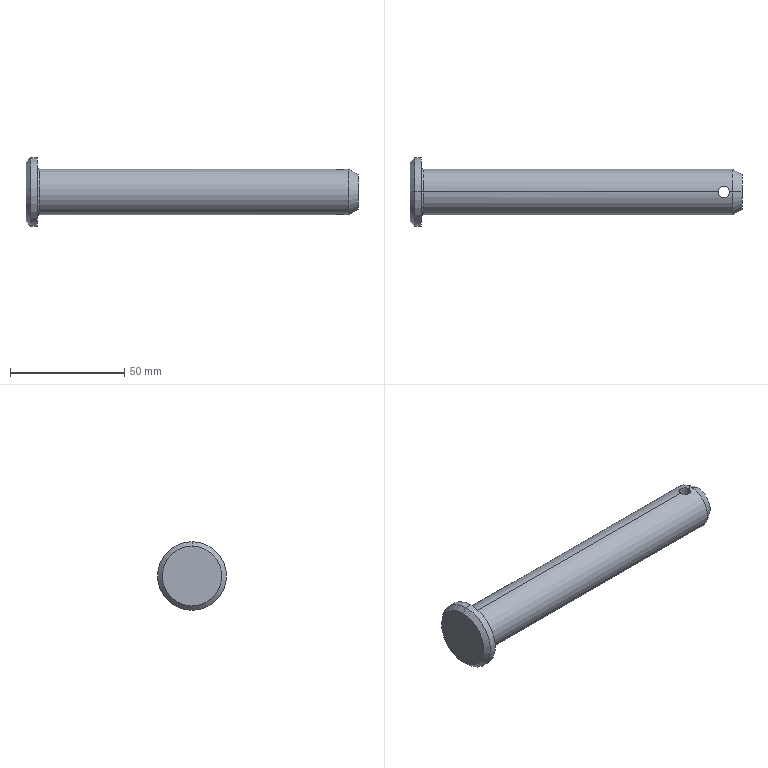Part | SolidWorks | features Chamfer 1, Fillet 1, ICE 1, Revolution 1 | 1 solid | 15 faces | box 145 x 30 x 30 mm | volume 46693 mm3 | cylinder 6 | cone 4 | plane 3 | torus 2 | commonest cylinder face diameters 5 x2 20 x2 30 x2
STEP:
#1=CARTESIAN_POINT('',(145.,0.,-7.691));
#2=VERTEX_POINT('',#1);
#3=CARTESIAN_POINT('',(145.,0.,7.691));
#4=VERTEX_POINT('',#3);
#5=CARTESIAN_POINT('',(145.,0.,0.));
#6=DIRECTION('',(1.,0.,0.));
#7=DIRECTION('',(0.,0.,-1.));
#8=AXIS2_PLACEMENT_3D('',#5,#6,#7);
#9=CIRCLE('',#8,7.691);
#10=EDGE_CURVE('',#2,#4,#9,.T.);
#11=ORIENTED_EDGE('',*,*,#10,.F.);
#12=CARTESIAN_POINT('',(141.,0.,-10.));
#13=VERTEX_POINT('',#12);
#14=CARTESIAN_POINT('',(145.,0.,-7.691));
#15=DIRECTION('',(-0.866,0.,-0.5));
#16=VECTOR('',#15,1000.);
#17=LINE('',#14,#16);
#18=EDGE_CURVE('',#2,#13,#17,.T.);
#19=ORIENTED_EDGE('',*,*,#18,.T.);
#20=CARTESIAN_POINT('',(141.,0.,10.));
#21=VERTEX_POINT('',#20);
#22=CARTESIAN_POINT('',(141.,0.,0.));
#23=DIRECTION('',(-1.,0.,0.));
#24=DIRECTION('',(0.,0.,-1.));
#25=AXIS2_PLACEMENT_3D('',#22,#23,#24);
#26=CIRCLE('',#25,10.);
#27=EDGE_CURVE('',#21,#13,#26,.T.);
#28=ORIENTED_EDGE('',*,*,#27,.F.);
#29=CARTESIAN_POINT('',(145.,0.,7.691));
#30=DIRECTION('',(-0.866,0.,0.5));
#31=VECTOR('',#30,1000.);
#32=LINE('',#29,#31);
#33=EDGE_CURVE('',#4,#21,#32,.T.);
#34=ORIENTED_EDGE('',*,*,#33,.F.);
#35=EDGE_LOOP('',(#11,#19,#28,#34));
#36=FACE_OUTER_BOUND('',#35,.T.);
#37=CARTESIAN_POINT('',(145.,0.,0.));
#38=DIRECTION('',(-1.,0.,0.));
#39=DIRECTION('',(0.,0.,1.));
#40=AXIS2_PLACEMENT_3D('',#37,#38,#39);
#41=CONICAL_SURFACE('',#40,7.691,0.5236);
#42=ADVANCED_FACE('',(#36),#41,.T.);
#43=CARTESIAN_POINT('',(6.,0.,10.));
#44=VERTEX_POINT('',#43);
#45=CARTESIAN_POINT('',(6.,0.,-10.));
#46=VERTEX_POINT('',#45);
#47=CARTESIAN_POINT('',(6.,0.,0.));
#48=DIRECTION('',(1.,0.,0.));
#49=DIRECTION('',(0.,0.,-1.));
#50=AXIS2_PLACEMENT_3D('',#47,#48,#49);
#51=CIRCLE('',#50,10.);
#52=EDGE_CURVE('',#44,#46,#51,.T.);
#53=ORIENTED_EDGE('',*,*,#52,.F.);
#54=CARTESIAN_POINT('',(5.,0.,11.));
#55=VERTEX_POINT('',#54);
#56=CARTESIAN_POINT('',(6.,0.,11.));
#57=DIRECTION('',(0.,1.,0.));
#58=DIRECTION('',(0.,0.,1.));
#59=AXIS2_PLACEMENT_3D('',#56,#57,#58);
#60=CIRCLE('',#59,1.);
#61=EDGE_CURVE('',#44,#55,#60,.T.);
#62=ORIENTED_EDGE('',*,*,#61,.T.);
#63=CARTESIAN_POINT('',(5.,0.,-11.));
#64=VERTEX_POINT('',#63);
#65=CARTESIAN_POINT('',(5.,0.,0.));
#66=DIRECTION('',(-1.,0.,0.));
#67=DIRECTION('',(0.,0.,-1.));
#68=AXIS2_PLACEMENT_3D('',#65,#66,#67);
#69=CIRCLE('',#68,11.);
#70=EDGE_CURVE('',#64,#55,#69,.T.);
#71=ORIENTED_EDGE('',*,*,#70,.F.);
#72=CARTESIAN_POINT('',(6.,0.,-11.));
#73=DIRECTION('',(0.,-1.,0.));
#74=DIRECTION('',(0.,0.,-1.));
#75=AXIS2_PLACEMENT_3D('',#72,#73,#74);
#76=CIRCLE('',#75,1.);
#77=EDGE_CURVE('',#46,#64,#76,.T.);
#78=ORIENTED_EDGE('',*,*,#77,.F.);
#79=EDGE_LOOP('',(#53,#62,#71,#78));
#80=FACE_OUTER_BOUND('',#79,.T.);
#81=CARTESIAN_POINT('',(6.,0.,0.));
#82=DIRECTION('',(1.,0.,0.));
#83=DIRECTION('',(0.,0.,-1.));
#84=AXIS2_PLACEMENT_3D('',#81,#82,#83);
#85=TOROIDAL_SURFACE('',#84,11.,1.);
#86=ADVANCED_FACE('',(#80),#85,.F.);
#87=CARTESIAN_POINT('',(139.5,0.,-10.));
#88=VERTEX_POINT('',#87);
#89=CARTESIAN_POINT('',(134.5,0.,-10.));
#90=VERTEX_POINT('',#89);
#91=CARTESIAN_POINT('',(139.5,0.,-10.));
#92=CARTESIAN_POINT('',(139.5,-0.327,-10.));
#93=CARTESIAN_POINT('',(139.434,-0.6572,-9.983));
#94=CARTESIAN_POINT('',(139.247,-1.109,-9.939));
#95=CARTESIAN_POINT('',(139.168,-1.255,-9.922));
#96=CARTESIAN_POINT('',(138.987,-1.526,-9.884));
#97=CARTESIAN_POINT('',(138.884,-1.652,-9.863));
#98=CARTESIAN_POINT('',(138.653,-1.882,-9.822));
#99=CARTESIAN_POINT('',(138.525,-1.987,-9.801));
#100=CARTESIAN_POINT('',(138.255,-2.168,-9.763));
#101=CARTESIAN_POINT('',(138.112,-2.245,-9.745));
#102=CARTESIAN_POINT('',(137.808,-2.372,-9.715));
#103=CARTESIAN_POINT('',(137.651,-2.419,-9.703));
#104=CARTESIAN_POINT('',(137.331,-2.483,-9.687));
#105=CARTESIAN_POINT('',(137.166,-2.5,-9.682));
#106=CARTESIAN_POINT('',(136.836,-2.5,-9.682));
#107=CARTESIAN_POINT('',(136.673,-2.484,-9.687));
#108=CARTESIAN_POINT('',(136.352,-2.42,-9.703));
#109=CARTESIAN_POINT('',(136.193,-2.372,-9.715));
#110=CARTESIAN_POINT('',(135.891,-2.247,-9.745));
#111=CARTESIAN_POINT('',(135.747,-2.17,-9.762));
#112=CARTESIAN_POINT('',(135.475,-1.988,-9.801));
#113=CARTESIAN_POINT('',(135.348,-1.883,-9.822));
#114=CARTESIAN_POINT('',(135.118,-1.654,-9.863));
#115=CARTESIAN_POINT('',(135.014,-1.527,-9.884));
#116=CARTESIAN_POINT('',(134.832,-1.255,-9.922));
#117=CARTESIAN_POINT('',(134.755,-1.112,-9.939));
#118=CARTESIAN_POINT('',(134.629,-0.8107,-9.968));
#119=CARTESIAN_POINT('',(134.581,-0.6515,-9.98));
#120=CARTESIAN_POINT('',(134.516,-0.3293,-9.996));
#121=CARTESIAN_POINT('',(134.5,-0.1658,-10.));
#122=CARTESIAN_POINT('',(134.5,0.,-10.));
#123=B_SPLINE_CURVE_WITH_KNOTS('',3,(#91,#92,#93,#94,#95,#96,#97,#98,#99,#100,#101,#102,#103,#104,#105,#106,#107,#108,#109,#110,#111,#112,#113,#114,#115,#116,#117,#118,#119,#120,#121,#122),.UNSPECIFIED.,.F.,.F.,(4,2,2,2,2,2,2,2,2,2,2,2,2,2,2,4),(0.007847,0.008828,0.009318,0.009809,0.0103,0.01079,0.01128,0.01177,0.01226,0.01275,0.01324,0.01373,0.01422,0.01471,0.0152,0.01569),.UNSPECIFIED.);
#124=EDGE_CURVE('',#88,#90,#123,.T.);
#125=ORIENTED_EDGE('',*,*,#124,.T.);
#126=CARTESIAN_POINT('',(134.5,0.,10.));
#127=VERTEX_POINT('',#126);
#128=CARTESIAN_POINT('',(134.5,0.,-15.));
#129=DIRECTION('',(0.,0.,1.));
#130=VECTOR('',#129,1000.);
#131=LINE('',#128,#130);
#132=EDGE_CURVE('',#90,#127,#131,.T.);
#133=ORIENTED_EDGE('',*,*,#132,.T.);
#134=CARTESIAN_POINT('',(139.5,0.,10.));
#135=VERTEX_POINT('',#134);
#136=CARTESIAN_POINT('',(134.5,0.,10.));
#137=CARTESIAN_POINT('',(134.5,-0.327,10.));
#138=CARTESIAN_POINT('',(134.566,-0.6572,9.983));
#139=CARTESIAN_POINT('',(134.753,-1.109,9.939));
#140=CARTESIAN_POINT('',(134.832,-1.255,9.922));
#141=CARTESIAN_POINT('',(135.013,-1.526,9.884));
#142=CARTESIAN_POINT('',(135.116,-1.652,9.863));
#143=CARTESIAN_POINT('',(135.347,-1.882,9.822));
#144=CARTESIAN_POINT('',(135.475,-1.987,9.801));
#145=CARTESIAN_POINT('',(135.745,-2.168,9.763));
#146=CARTESIAN_POINT('',(135.888,-2.245,9.745));
#147=CARTESIAN_POINT('',(136.192,-2.372,9.715));
#148=CARTESIAN_POINT('',(136.349,-2.419,9.703));
#149=CARTESIAN_POINT('',(136.669,-2.483,9.687));
#150=CARTESIAN_POINT('',(136.834,-2.5,9.682));
#151=CARTESIAN_POINT('',(137.164,-2.5,9.682));
#152=CARTESIAN_POINT('',(137.327,-2.484,9.687));
#153=CARTESIAN_POINT('',(137.648,-2.42,9.703));
#154=CARTESIAN_POINT('',(137.807,-2.372,9.715));
#155=CARTESIAN_POINT('',(138.109,-2.247,9.745));
#156=CARTESIAN_POINT('',(138.253,-2.17,9.762));
#157=CARTESIAN_POINT('',(138.525,-1.988,9.801));
#158=CARTESIAN_POINT('',(138.652,-1.883,9.822));
#159=CARTESIAN_POINT('',(138.882,-1.654,9.863));
#160=CARTESIAN_POINT('',(138.986,-1.527,9.884));
#161=CARTESIAN_POINT('',(139.168,-1.255,9.922));
#162=CARTESIAN_POINT('',(139.245,-1.112,9.939));
#163=CARTESIAN_POINT('',(139.371,-0.8107,9.968));
#164=CARTESIAN_POINT('',(139.419,-0.6515,9.98));
#165=CARTESIAN_POINT('',(139.484,-0.3293,9.996));
#166=CARTESIAN_POINT('',(139.5,-0.1658,10.));
#167=CARTESIAN_POINT('',(139.5,0.,10.));
#168=B_SPLINE_CURVE_WITH_KNOTS('',3,(#136,#137,#138,#139,#140,#141,#142,#143,#144,#145,#146,#147,#148,#149,#150,#151,#152,#153,#154,#155,#156,#157,#158,#159,#160,#161,#162,#163,#164,#165,#166,#167),.UNSPECIFIED.,.F.,.F.,(4,2,2,2,2,2,2,2,2,2,2,2,2,2,2,4),(0.007847,0.008828,0.009318,0.009809,0.0103,0.01079,0.01128,0.01177,0.01226,0.01275,0.01324,0.01373,0.01422,0.01471,0.0152,0.01569),.UNSPECIFIED.);
#169=EDGE_CURVE('',#127,#135,#168,.T.);
#170=ORIENTED_EDGE('',*,*,#169,.T.);
#171=CARTESIAN_POINT('',(139.5,0.,-15.));
#172=DIRECTION('',(0.,0.,1.));
#173=VECTOR('',#172,1000.);
#174=LINE('',#171,#173);
#175=EDGE_CURVE('',#88,#135,#174,.T.);
#176=ORIENTED_EDGE('',*,*,#175,.F.);
#177=EDGE_LOOP('',(#125,#133,#170,#176));
#178=FACE_OUTER_BOUND('',#177,.T.);
#179=CARTESIAN_POINT('',(137.,0.,-15.));
#180=DIRECTION('',(0.,0.,1.));
#181=DIRECTION('',(1.,0.,0.));
#182=AXIS2_PLACEMENT_3D('',#179,#180,#181);
#183=CYLINDRICAL_SURFACE('',#182,2.5);
#184=ADVANCED_FACE('',(#178),#183,.F.);
#185=CARTESIAN_POINT('',(6.,0.,0.));
#186=DIRECTION('',(1.,0.,0.));
#187=DIRECTION('',(0.,0.,-1.));
#188=AXIS2_PLACEMENT_3D('',#185,#186,#187);
#189=CIRCLE('',#188,10.);
#190=EDGE_CURVE('',#46,#44,#189,.T.);
#191=ORIENTED_EDGE('',*,*,#190,.T.);
#192=CARTESIAN_POINT('',(0.,0.,10.));
#193=DIRECTION('',(1.,0.,0.));
#194=VECTOR('',#193,1000.);
#195=LINE('',#192,#194);
#196=EDGE_CURVE('',#44,#127,#195,.T.);
#197=ORIENTED_EDGE('',*,*,#196,.T.);
#198=CARTESIAN_POINT('',(139.5,0.,10.));
#199=CARTESIAN_POINT('',(139.5,0.1659,10.));
#200=CARTESIAN_POINT('',(139.484,0.3289,9.996));
#201=CARTESIAN_POINT('',(139.42,0.6493,9.98));
#202=CARTESIAN_POINT('',(139.371,0.8085,9.968));
#203=CARTESIAN_POINT('',(139.246,1.111,9.939));
#204=CARTESIAN_POINT('',(139.169,1.254,9.922));
#205=CARTESIAN_POINT('',(138.987,1.526,9.884));
#206=CARTESIAN_POINT('',(138.882,1.654,9.863));
#207=CARTESIAN_POINT('',(138.538,1.998,9.801));
#208=CARTESIAN_POINT('',(138.26,2.184,9.759));
#209=CARTESIAN_POINT('',(137.809,2.371,9.715));
#210=CARTESIAN_POINT('',(137.651,2.419,9.703));
#211=CARTESIAN_POINT('',(137.328,2.484,9.687));
#212=CARTESIAN_POINT('',(137.165,2.5,9.682));
#213=CARTESIAN_POINT('',(136.837,2.5,9.682));
#214=CARTESIAN_POINT('',(136.671,2.484,9.687));
#215=CARTESIAN_POINT('',(136.35,2.419,9.703));
#216=CARTESIAN_POINT('',(136.193,2.372,9.715));
#217=CARTESIAN_POINT('',(135.738,2.183,9.76));
#218=CARTESIAN_POINT('',(135.463,1.999,9.801));
#219=CARTESIAN_POINT('',(135.116,1.652,9.863));
#220=CARTESIAN_POINT('',(135.013,1.526,9.884));
#221=CARTESIAN_POINT('',(134.832,1.256,9.922));
#222=CARTESIAN_POINT('',(134.754,1.109,9.939));
#223=CARTESIAN_POINT('',(134.628,0.8074,9.969));
#224=CARTESIAN_POINT('',(134.581,0.6515,9.98));
#225=CARTESIAN_POINT('',(134.516,0.3295,9.996));
#226=CARTESIAN_POINT('',(134.5,0.1635,10.));
#227=CARTESIAN_POINT('',(134.5,0.,10.));
#228=B_SPLINE_CURVE_WITH_KNOTS('',3,(#198,#199,#200,#201,#202,#203,#204,#205,#206,#207,#208,#209,#210,#211,#212,#213,#214,#215,#216,#217,#218,#219,#220,#221,#222,#223,#224,#225,#226,#227),.UNSPECIFIED.,.F.,.F.,(4,2,2,2,2,2,2,2,2,2,2,2,2,2,4),(0.,0.0004905,0.0009809,0.001471,0.001962,0.002943,0.003433,0.003924,0.004414,0.004905,0.005886,0.006376,0.006866,0.007357,0.007847),.UNSPECIFIED.);
#229=EDGE_CURVE('',#135,#127,#228,.T.);
#230=ORIENTED_EDGE('',*,*,#229,.F.);
#231=CARTESIAN_POINT('',(0.,0.,10.));
#232=DIRECTION('',(1.,0.,0.));
#233=VECTOR('',#232,1000.);
#234=LINE('',#231,#233);
#235=EDGE_CURVE('',#135,#21,#234,.T.);
#236=ORIENTED_EDGE('',*,*,#235,.T.);
#237=ORIENTED_EDGE('',*,*,#27,.T.);
#238=CARTESIAN_POINT('',(0.,0.,-10.));
#239=DIRECTION('',(1.,0.,0.));
#240=VECTOR('',#239,1000.);
#241=LINE('',#238,#240);
#242=EDGE_CURVE('',#88,#13,#241,.T.);
#243=ORIENTED_EDGE('',*,*,#242,.F.);
#244=CARTESIAN_POINT('',(134.5,0.,-10.));
#245=CARTESIAN_POINT('',(134.5,0.1659,-10.));
#246=CARTESIAN_POINT('',(134.516,0.3289,-9.996));
#247=CARTESIAN_POINT('',(134.58,0.6493,-9.98));
#248=CARTESIAN_POINT('',(134.629,0.8085,-9.968));
#249=CARTESIAN_POINT('',(134.754,1.111,-9.939));
#250=CARTESIAN_POINT('',(134.831,1.254,-9.922));
#251=CARTESIAN_POINT('',(135.013,1.526,-9.884));
#252=CARTESIAN_POINT('',(135.118,1.654,-9.863));
#253=CARTESIAN_POINT('',(135.462,1.998,-9.801));
#254=CARTESIAN_POINT('',(135.74,2.184,-9.759));
#255=CARTESIAN_POINT('',(136.191,2.371,-9.715));
#256=CARTESIAN_POINT('',(136.349,2.419,-9.703));
#257=CARTESIAN_POINT('',(136.672,2.484,-9.687));
#258=CARTESIAN_POINT('',(136.835,2.5,-9.682));
#259=CARTESIAN_POINT('',(137.163,2.5,-9.682));
#260=CARTESIAN_POINT('',(137.329,2.484,-9.687));
#261=CARTESIAN_POINT('',(137.65,2.419,-9.703));
#262=CARTESIAN_POINT('',(137.807,2.372,-9.715));
#263=CARTESIAN_POINT('',(138.262,2.183,-9.76));
#264=CARTESIAN_POINT('',(138.537,1.999,-9.801));
#265=CARTESIAN_POINT('',(138.884,1.652,-9.863));
#266=CARTESIAN_POINT('',(138.987,1.526,-9.884));
#267=CARTESIAN_POINT('',(139.168,1.256,-9.922));
#268=CARTESIAN_POINT('',(139.246,1.109,-9.939));
#269=CARTESIAN_POINT('',(139.372,0.8074,-9.969));
#270=CARTESIAN_POINT('',(139.419,0.6515,-9.98));
#271=CARTESIAN_POINT('',(139.484,0.3295,-9.996));
#272=CARTESIAN_POINT('',(139.5,0.1635,-10.));
#273=CARTESIAN_POINT('',(139.5,0.,-10.));
#274=B_SPLINE_CURVE_WITH_KNOTS('',3,(#244,#245,#246,#247,#248,#249,#250,#251,#252,#253,#254,#255,#256,#257,#258,#259,#260,#261,#262,#263,#264,#265,#266,#267,#268,#269,#270,#271,#272,#273),.UNSPECIFIED.,.F.,.F.,(4,2,2,2,2,2,2,2,2,2,2,2,2,2,4),(0.,0.0004905,0.0009809,0.001471,0.001962,0.002943,0.003433,0.003924,0.004414,0.004905,0.005886,0.006376,0.006866,0.007357,0.007847),.UNSPECIFIED.);
#275=EDGE_CURVE('',#90,#88,#274,.T.);
#276=ORIENTED_EDGE('',*,*,#275,.F.);
#277=CARTESIAN_POINT('',(0.,0.,-10.));
#278=DIRECTION('',(1.,0.,0.));
#279=VECTOR('',#278,1000.);
#280=LINE('',#277,#279);
#281=EDGE_CURVE('',#46,#90,#280,.T.);
#282=ORIENTED_EDGE('',*,*,#281,.F.);
#283=EDGE_LOOP('',(#191,#197,#230,#236,#237,#243,#276,#282));
#284=FACE_OUTER_BOUND('',#283,.T.);
#285=CARTESIAN_POINT('',(0.,0.,0.));
#286=DIRECTION('',(1.,0.,0.));
#287=DIRECTION('',(0.,0.,-1.));
#288=AXIS2_PLACEMENT_3D('',#285,#286,#287);
#289=CYLINDRICAL_SURFACE('',#288,10.);
#290=ADVANCED_FACE('',(#284),#289,.T.);
#291=CARTESIAN_POINT('',(2.,0.,-15.));
#292=VERTEX_POINT('',#291);
#293=CARTESIAN_POINT('',(2.,0.,15.));
#294=VERTEX_POINT('',#293);
#295=CARTESIAN_POINT('',(2.,0.,0.));
#296=DIRECTION('',(1.,0.,0.));
#297=DIRECTION('',(0.,0.,-1.));
#298=AXIS2_PLACEMENT_3D('',#295,#296,#297);
#299=CIRCLE('',#298,15.);
#300=EDGE_CURVE('',#292,#294,#299,.T.);
#301=ORIENTED_EDGE('',*,*,#300,.T.);
#302=CARTESIAN_POINT('',(5.,0.,15.));
#303=VERTEX_POINT('',#302);
#304=CARTESIAN_POINT('',(0.,0.,15.));
#305=DIRECTION('',(1.,0.,0.));
#306=VECTOR('',#305,1000.);
#307=LINE('',#304,#306);
#308=EDGE_CURVE('',#294,#303,#307,.T.);
#309=ORIENTED_EDGE('',*,*,#308,.T.);
#310=CARTESIAN_POINT('',(5.,0.,-15.));
#311=VERTEX_POINT('',#310);
#312=CARTESIAN_POINT('',(5.,0.,0.));
#313=DIRECTION('',(1.,0.,0.));
#314=DIRECTION('',(0.,0.,-1.));
#315=AXIS2_PLACEMENT_3D('',#312,#313,#314);
#316=CIRCLE('',#315,15.);
#317=EDGE_CURVE('',#311,#303,#316,.T.);
#318=ORIENTED_EDGE('',*,*,#317,.F.);
#319=CARTESIAN_POINT('',(0.,0.,-15.));
#320=DIRECTION('',(1.,0.,0.));
#321=VECTOR('',#320,1000.);
#322=LINE('',#319,#321);
#323=EDGE_CURVE('',#292,#311,#322,.T.);
#324=ORIENTED_EDGE('',*,*,#323,.F.);
#325=EDGE_LOOP('',(#301,#309,#318,#324));
#326=FACE_OUTER_BOUND('',#325,.T.);
#327=CARTESIAN_POINT('',(0.,0.,0.));
#328=DIRECTION('',(1.,0.,0.));
#329=DIRECTION('',(0.,0.,-1.));
#330=AXIS2_PLACEMENT_3D('',#327,#328,#329);
#331=CYLINDRICAL_SURFACE('',#330,15.);
#332=ADVANCED_FACE('',(#326),#331,.T.);
#333=CARTESIAN_POINT('',(0.,0.,-13.));
#334=VERTEX_POINT('',#333);
#335=CARTESIAN_POINT('',(0.,0.,13.));
#336=VERTEX_POINT('',#335);
#337=CARTESIAN_POINT('',(0.,0.,0.));
#338=DIRECTION('',(1.,0.,0.));
#339=DIRECTION('',(0.,0.,-1.));
#340=AXIS2_PLACEMENT_3D('',#337,#338,#339);
#341=CIRCLE('',#340,13.);
#342=EDGE_CURVE('',#334,#336,#341,.T.);
#343=ORIENTED_EDGE('',*,*,#342,.T.);
#344=CARTESIAN_POINT('',(2.,0.,15.));
#345=DIRECTION('',(0.7071,0.,0.7071));
#346=VECTOR('',#345,1000.);
#347=LINE('',#344,#346);
#348=EDGE_CURVE('',#336,#294,#347,.T.);
#349=ORIENTED_EDGE('',*,*,#348,.T.);
#350=ORIENTED_EDGE('',*,*,#300,.F.);
#351=CARTESIAN_POINT('',(2.,0.,-15.));
#352=DIRECTION('',(0.7071,0.,-0.7071));
#353=VECTOR('',#352,1000.);
#354=LINE('',#351,#353);
#355=EDGE_CURVE('',#334,#292,#354,.T.);
#356=ORIENTED_EDGE('',*,*,#355,.F.);
#357=EDGE_LOOP('',(#343,#349,#350,#356));
#358=FACE_OUTER_BOUND('',#357,.T.);
#359=CARTESIAN_POINT('',(2.,0.,0.));
#360=DIRECTION('',(1.,0.,0.));
#361=DIRECTION('',(0.,0.,-1.));
#362=AXIS2_PLACEMENT_3D('',#359,#360,#361);
#363=CONICAL_SURFACE('',#362,15.,0.7854);
#364=ADVANCED_FACE('',(#358),#363,.T.);
#365=ORIENTED_EDGE('',*,*,#342,.F.);
#366=CARTESIAN_POINT('',(0.,0.,0.));
#367=DIRECTION('',(1.,0.,0.));
#368=DIRECTION('',(0.,0.,-1.));
#369=AXIS2_PLACEMENT_3D('',#366,#367,#368);
#370=CIRCLE('',#369,13.);
#371=EDGE_CURVE('',#336,#334,#370,.T.);
#372=ORIENTED_EDGE('',*,*,#371,.F.);
#373=EDGE_LOOP('',(#365,#372));
#374=FACE_OUTER_BOUND('',#373,.T.);
#375=CARTESIAN_POINT('',(0.,0.,0.));
#376=DIRECTION('',(-1.,0.,0.));
#377=DIRECTION('',(0.,0.,1.));
#378=AXIS2_PLACEMENT_3D('',#375,#376,#377);
#379=PLANE('',#378);
#380=ADVANCED_FACE('',(#374),#379,.T.);
#381=ORIENTED_EDGE('',*,*,#348,.F.);
#382=ORIENTED_EDGE('',*,*,#371,.T.);
#383=ORIENTED_EDGE('',*,*,#355,.T.);
#384=CARTESIAN_POINT('',(2.,0.,0.));
#385=DIRECTION('',(1.,0.,0.));
#386=DIRECTION('',(0.,0.,-1.));
#387=AXIS2_PLACEMENT_3D('',#384,#385,#386);
#388=CIRCLE('',#387,15.);
#389=EDGE_CURVE('',#294,#292,#388,.T.);
#390=ORIENTED_EDGE('',*,*,#389,.F.);
#391=EDGE_LOOP('',(#381,#382,#383,#390));
#392=FACE_OUTER_BOUND('',#391,.T.);
#393=CARTESIAN_POINT('',(2.,0.,0.));
#394=DIRECTION('',(1.,0.,0.));
#395=DIRECTION('',(0.,0.,-1.));
#396=AXIS2_PLACEMENT_3D('',#393,#394,#395);
#397=CONICAL_SURFACE('',#396,15.,0.7854);
#398=ADVANCED_FACE('',(#392),#397,.T.);
#399=ORIENTED_EDGE('',*,*,#308,.F.);
#400=ORIENTED_EDGE('',*,*,#389,.T.);
#401=ORIENTED_EDGE('',*,*,#323,.T.);
#402=CARTESIAN_POINT('',(5.,0.,0.));
#403=DIRECTION('',(1.,0.,0.));
#404=DIRECTION('',(0.,0.,-1.));
#405=AXIS2_PLACEMENT_3D('',#402,#403,#404);
#406=CIRCLE('',#405,15.);
#407=EDGE_CURVE('',#303,#311,#406,.T.);
#408=ORIENTED_EDGE('',*,*,#407,.F.);
#409=EDGE_LOOP('',(#399,#400,#401,#408));
#410=FACE_OUTER_BOUND('',#409,.T.);
#411=CARTESIAN_POINT('',(0.,0.,0.));
#412=DIRECTION('',(1.,0.,0.));
#413=DIRECTION('',(0.,0.,-1.));
#414=AXIS2_PLACEMENT_3D('',#411,#412,#413);
#415=CYLINDRICAL_SURFACE('',#414,15.);
#416=ADVANCED_FACE('',(#410),#415,.T.);
#417=ORIENTED_EDGE('',*,*,#70,.T.);
#418=CARTESIAN_POINT('',(5.,0.,0.));
#419=DIRECTION('',(-1.,0.,0.));
#420=DIRECTION('',(0.,0.,-1.));
#421=AXIS2_PLACEMENT_3D('',#418,#419,#420);
#422=CIRCLE('',#421,11.);
#423=EDGE_CURVE('',#55,#64,#422,.T.);
#424=ORIENTED_EDGE('',*,*,#423,.T.);
#425=EDGE_LOOP('',(#417,#424));
#426=FACE_BOUND('',#425,.T.);
#427=ORIENTED_EDGE('',*,*,#317,.T.);
#428=ORIENTED_EDGE('',*,*,#407,.T.);
#429=EDGE_LOOP('',(#427,#428));
#430=FACE_OUTER_BOUND('',#429,.T.);
#431=CARTESIAN_POINT('',(5.,15.,0.));
#432=DIRECTION('',(1.,0.,0.));
#433=DIRECTION('',(0.,0.,-1.));
#434=AXIS2_PLACEMENT_3D('',#431,#432,#433);
#435=PLANE('',#434);
#436=ADVANCED_FACE('',(#426,#430),#435,.T.);
#437=ORIENTED_EDGE('',*,*,#196,.F.);
#438=ORIENTED_EDGE('',*,*,#52,.T.);
#439=ORIENTED_EDGE('',*,*,#281,.T.);
#440=ORIENTED_EDGE('',*,*,#124,.F.);
#441=ORIENTED_EDGE('',*,*,#242,.T.);
#442=CARTESIAN_POINT('',(141.,0.,0.));
#443=DIRECTION('',(-1.,0.,0.));
#444=DIRECTION('',(0.,0.,-1.));
#445=AXIS2_PLACEMENT_3D('',#442,#443,#444);
#446=CIRCLE('',#445,10.);
#447=EDGE_CURVE('',#13,#21,#446,.T.);
#448=ORIENTED_EDGE('',*,*,#447,.T.);
#449=ORIENTED_EDGE('',*,*,#235,.F.);
#450=ORIENTED_EDGE('',*,*,#169,.F.);
#451=EDGE_LOOP('',(#437,#438,#439,#440,#441,#448,#449,#450));
#452=FACE_OUTER_BOUND('',#451,.T.);
#453=CARTESIAN_POINT('',(0.,0.,0.));
#454=DIRECTION('',(1.,0.,0.));
#455=DIRECTION('',(0.,0.,-1.));
#456=AXIS2_PLACEMENT_3D('',#453,#454,#455);
#457=CYLINDRICAL_SURFACE('',#456,10.);
#458=ADVANCED_FACE('',(#452),#457,.T.);
#459=CARTESIAN_POINT('',(145.,0.,0.));
#460=DIRECTION('',(1.,0.,0.));
#461=DIRECTION('',(0.,0.,-1.));
#462=AXIS2_PLACEMENT_3D('',#459,#460,#461);
#463=CIRCLE('',#462,7.691);
#464=EDGE_CURVE('',#4,#2,#463,.T.);
#465=ORIENTED_EDGE('',*,*,#464,.T.);
#466=ORIENTED_EDGE('',*,*,#10,.T.);
#467=EDGE_LOOP('',(#465,#466));
#468=FACE_OUTER_BOUND('',#467,.T.);
#469=CARTESIAN_POINT('',(145.,10.,0.));
#470=DIRECTION('',(1.,0.,0.));
#471=DIRECTION('',(0.,0.,-1.));
#472=AXIS2_PLACEMENT_3D('',#469,#470,#471);
#473=PLANE('',#472);
#474=ADVANCED_FACE('',(#468),#473,.T.);
#475=ORIENTED_EDGE('',*,*,#132,.F.);
#476=ORIENTED_EDGE('',*,*,#275,.T.);
#477=ORIENTED_EDGE('',*,*,#175,.T.);
#478=ORIENTED_EDGE('',*,*,#229,.T.);
#479=EDGE_LOOP('',(#475,#476,#477,#478));
#480=FACE_OUTER_BOUND('',#479,.T.);
#481=CARTESIAN_POINT('',(137.,0.,-15.));
#482=DIRECTION('',(0.,0.,1.));
#483=DIRECTION('',(1.,0.,0.));
#484=AXIS2_PLACEMENT_3D('',#481,#482,#483);
#485=CYLINDRICAL_SURFACE('',#484,2.5);
#486=ADVANCED_FACE('',(#480),#485,.F.);
#487=ORIENTED_EDGE('',*,*,#61,.F.);
#488=ORIENTED_EDGE('',*,*,#190,.F.);
#489=ORIENTED_EDGE('',*,*,#77,.T.);
#490=ORIENTED_EDGE('',*,*,#423,.F.);
#491=EDGE_LOOP('',(#487,#488,#489,#490));
#492=FACE_OUTER_BOUND('',#491,.T.);
#493=CARTESIAN_POINT('',(6.,0.,0.));
#494=DIRECTION('',(1.,0.,0.));
#495=DIRECTION('',(0.,0.,-1.));
#496=AXIS2_PLACEMENT_3D('',#493,#494,#495);
#497=TOROIDAL_SURFACE('',#496,11.,1.);
#498=ADVANCED_FACE('',(#492),#497,.F.);
#499=ORIENTED_EDGE('',*,*,#18,.F.);
#500=ORIENTED_EDGE('',*,*,#464,.F.);
#501=ORIENTED_EDGE('',*,*,#33,.T.);
#502=ORIENTED_EDGE('',*,*,#447,.F.);
#503=EDGE_LOOP('',(#499,#500,#501,#502));
#504=FACE_OUTER_BOUND('',#503,.T.);
#505=CARTESIAN_POINT('',(145.,0.,0.));
#506=DIRECTION('',(-1.,0.,0.));
#507=DIRECTION('',(0.,0.,1.));
#508=AXIS2_PLACEMENT_3D('',#505,#506,#507);
#509=CONICAL_SURFACE('',#508,7.691,0.5236);
#510=ADVANCED_FACE('',(#504),#509,.T.);
#511=CLOSED_SHELL('',(#42,#86,#184,#290,#332,#364,#380,#398,#416,#436,#458,#474,#486,#498,#510));
#512=MANIFOLD_SOLID_BREP('',#511);
#513=CARTESIAN_POINT('',(0.,0.,0.));
#514=DIRECTION('',(0.,0.,1.));
#515=DIRECTION('',(1.,0.,0.));
#516=AXIS2_PLACEMENT_3D('',#513,#514,#515);
#517=(LENGTH_UNIT()NAMED_UNIT(*)SI_UNIT(.MILLI.,.METRE.));
#518=UNCERTAINTY_MEASURE_WITH_UNIT(LENGTH_MEASURE(0.00001),#517,'','');
#519=(NAMED_UNIT(*)PLANE_ANGLE_UNIT()SI_UNIT($,.RADIAN.));
#520=(NAMED_UNIT(*)SI_UNIT($,.STERADIAN.)SOLID_ANGLE_UNIT());
#521=(GEOMETRIC_REPRESENTATION_CONTEXT(3)GLOBAL_UNCERTAINTY_ASSIGNED_CONTEXT((#518))GLOBAL_UNIT_ASSIGNED_CONTEXT((#517,#519,#520))REPRESENTATION_CONTEXT('',''));
#522=ADVANCED_BREP_SHAPE_REPRESENTATION('',(#512,#516),#521);